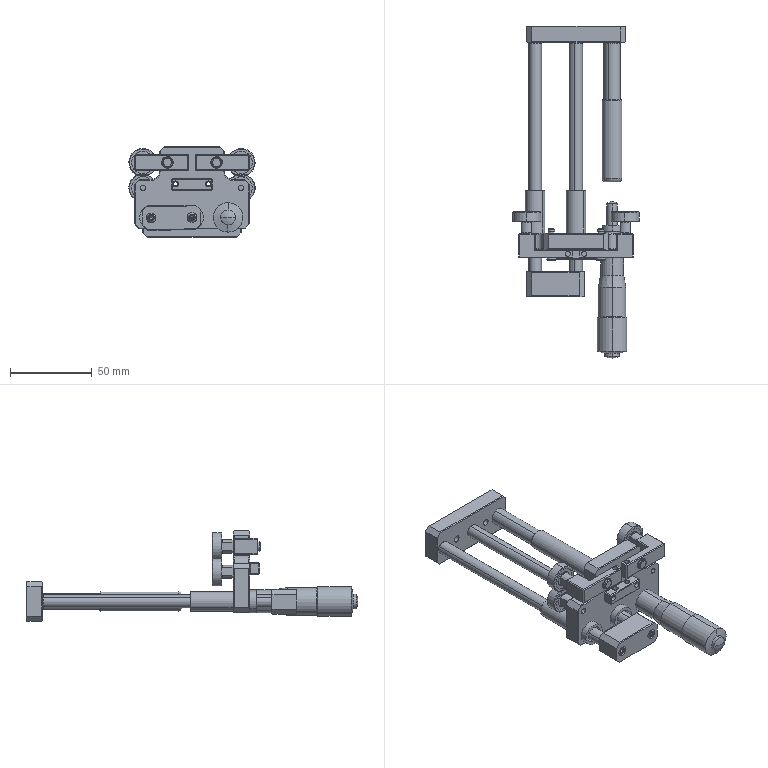Part | SolidWorks | features CompositeCurve 4, MateUpdatePoint 3 | 30 solids | 839 faces | box 77 x 202.46 x 55 mm | volume 99143 mm3 | cylinder 348 | plane 295 | cone 144 | torus 36 | spline 12 | sphere 4 | commonest cylinder face diameters 4 x76 6 x28 3.3 x24 8 x24 7 x20 5.15 x16